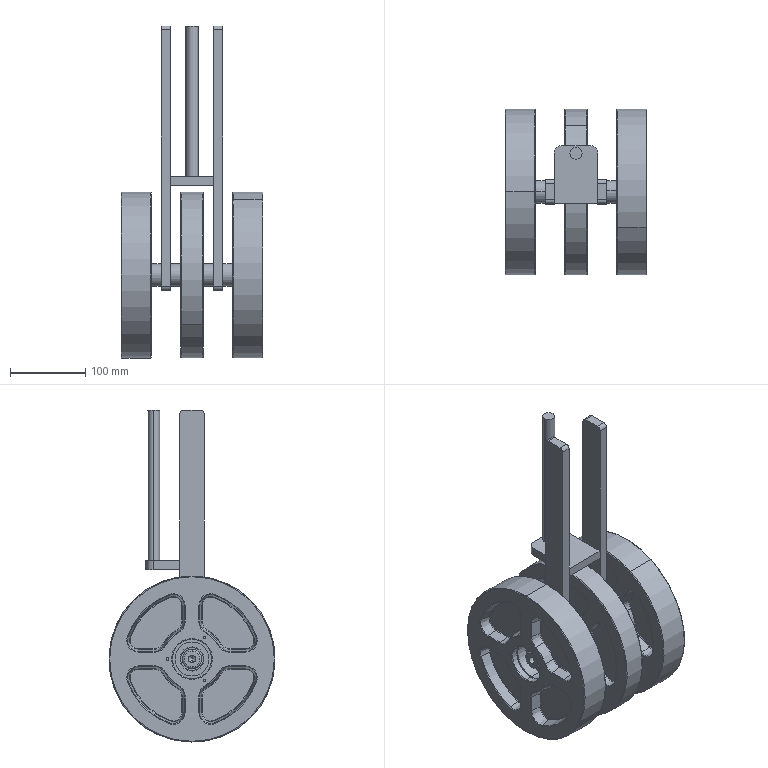Part | SolidWorks | features CompositeCurve 4 | 12 solids | 805 faces | box 188 x 220 x 440 mm | volume 3274270 mm3 | torus 340 | cylinder 188 | cone 148 | plane 129 | commonest cylinder face diameters 2 x96 3 x18 52 x12 10 x8 26 x8 30 x8